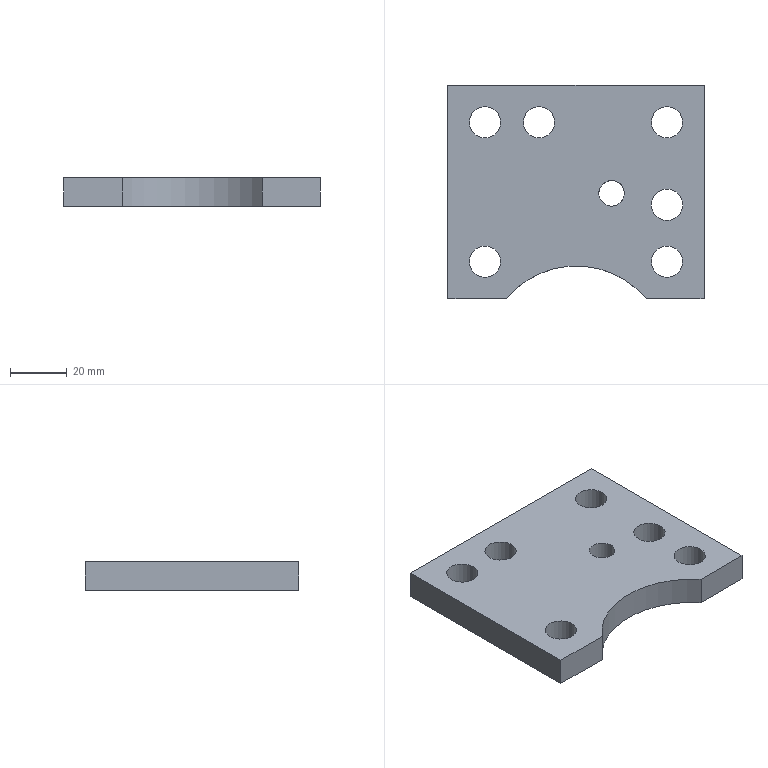Part | STEP file | PN_0043_id890_x_t | 1 solid | 15 faces | box 90 x 75 x 10 mm | volume 57234 mm3 | cylinder 8 | plane 7 | commonest cylinder face diameters 11 x6 9 x1 64 x1
STEP:
#1=CARTESIAN_POINT('',(-219.571,-141.5,105.));
#2=VERTEX_POINT('',#1);
#3=CARTESIAN_POINT('',(-219.571,-141.5,95.));
#4=VERTEX_POINT('',#3);
#5=CARTESIAN_POINT('',(-219.571,-141.5,96.5));
#6=DIRECTION('',(0.,0.,-1.));
#7=VECTOR('',#6,1.);
#8=LINE('',#5,#7);
#9=EDGE_CURVE('',#2,#4,#8,.T.);
#10=ORIENTED_EDGE('',*,*,#9,.F.);
#11=CARTESIAN_POINT('',(-240.086,-141.5,105.));
#12=VERTEX_POINT('',#11);
#13=CARTESIAN_POINT('',(-207.586,-141.5,105.));
#14=DIRECTION('',(-1.,0.,0.));
#15=VECTOR('',#14,1.);
#16=LINE('',#13,#15);
#17=EDGE_CURVE('',#2,#12,#16,.T.);
#18=ORIENTED_EDGE('',*,*,#17,.T.);
#19=CARTESIAN_POINT('',(-240.086,-141.5,95.));
#20=VERTEX_POINT('',#19);
#21=CARTESIAN_POINT('',(-240.086,-141.5,105.));
#22=DIRECTION('',(0.,0.,1.));
#23=VECTOR('',#22,1.);
#24=LINE('',#21,#23);
#25=EDGE_CURVE('',#20,#12,#24,.T.);
#26=ORIENTED_EDGE('',*,*,#25,.F.);
#27=CARTESIAN_POINT('',(-207.586,-141.5,95.));
#28=DIRECTION('',(1.,0.,0.));
#29=VECTOR('',#28,1.);
#30=LINE('',#27,#29);
#31=EDGE_CURVE('',#20,#4,#30,.T.);
#32=ORIENTED_EDGE('',*,*,#31,.T.);
#33=EDGE_LOOP('',(#10,#18,#26,#32));
#34=FACE_OUTER_BOUND('',#33,.T.);
#35=CARTESIAN_POINT('',(-207.586,-141.5,105.));
#36=DIRECTION('',(0.,-1.,0.));
#37=DIRECTION('',(0.,0.,-1.));
#38=AXIS2_PLACEMENT_3D('',#35,#36,#37);
#39=PLANE('',#38);
#40=ADVANCED_FACE('',(#34),#39,.T.);
#41=CARTESIAN_POINT('',(-221.586,-79.5,105.));
#42=VERTEX_POINT('',#41);
#43=CARTESIAN_POINT('',(-227.086,-79.5,105.));
#44=DIRECTION('',(0.,0.,1.));
#45=DIRECTION('',(1.,0.,0.));
#46=AXIS2_PLACEMENT_3D('',#43,#44,#45);
#47=CIRCLE('',#46,5.5);
#48=EDGE_CURVE('',#42,#42,#47,.T.);
#49=ORIENTED_EDGE('',*,*,#48,.F.);
#50=EDGE_LOOP('',(#49));
#51=FACE_BOUND('',#50,.T.);
#52=CARTESIAN_POINT('',(-202.586,-79.5,105.));
#53=VERTEX_POINT('',#52);
#54=CARTESIAN_POINT('',(-208.086,-79.5,105.));
#55=DIRECTION('',(0.,0.,-1.));
#56=DIRECTION('',(1.,0.,0.));
#57=AXIS2_PLACEMENT_3D('',#54,#55,#56);
#58=CIRCLE('',#57,5.5);
#59=EDGE_CURVE('',#53,#53,#58,.T.);
#60=ORIENTED_EDGE('',*,*,#59,.T.);
#61=EDGE_LOOP('',(#60));
#62=FACE_BOUND('',#61,.T.);
#63=CARTESIAN_POINT('',(-168.586,-79.5,105.));
#64=VERTEX_POINT('',#63);
#65=CARTESIAN_POINT('',(-163.086,-79.5,105.));
#66=DIRECTION('',(0.,0.,-1.));
#67=DIRECTION('',(-1.,0.,0.));
#68=AXIS2_PLACEMENT_3D('',#65,#66,#67);
#69=CIRCLE('',#68,5.5);
#70=EDGE_CURVE('',#64,#64,#69,.T.);
#71=ORIENTED_EDGE('',*,*,#70,.T.);
#72=EDGE_LOOP('',(#71));
#73=FACE_BOUND('',#72,.T.);
#74=CARTESIAN_POINT('',(-221.586,-128.5,105.));
#75=VERTEX_POINT('',#74);
#76=CARTESIAN_POINT('',(-227.086,-128.5,105.));
#77=DIRECTION('',(0.,0.,-1.));
#78=DIRECTION('',(1.,0.,0.));
#79=AXIS2_PLACEMENT_3D('',#76,#77,#78);
#80=CIRCLE('',#79,5.5);
#81=EDGE_CURVE('',#75,#75,#80,.T.);
#82=ORIENTED_EDGE('',*,*,#81,.T.);
#83=EDGE_LOOP('',(#82));
#84=FACE_BOUND('',#83,.T.);
#85=CARTESIAN_POINT('',(-168.586,-108.5,105.));
#86=VERTEX_POINT('',#85);
#87=CARTESIAN_POINT('',(-163.086,-108.5,105.));
#88=DIRECTION('',(0.,0.,-1.));
#89=DIRECTION('',(-1.,0.,0.));
#90=AXIS2_PLACEMENT_3D('',#87,#88,#89);
#91=CIRCLE('',#90,5.5);
#92=EDGE_CURVE('',#86,#86,#91,.T.);
#93=ORIENTED_EDGE('',*,*,#92,.T.);
#94=EDGE_LOOP('',(#93));
#95=FACE_BOUND('',#94,.T.);
#96=CARTESIAN_POINT('',(-168.586,-128.5,105.));
#97=VERTEX_POINT('',#96);
#98=CARTESIAN_POINT('',(-163.086,-128.5,105.));
#99=DIRECTION('',(0.,0.,1.));
#100=DIRECTION('',(-1.,0.,0.));
#101=AXIS2_PLACEMENT_3D('',#98,#99,#100);
#102=CIRCLE('',#101,5.5);
#103=EDGE_CURVE('',#97,#97,#102,.T.);
#104=ORIENTED_EDGE('',*,*,#103,.F.);
#105=EDGE_LOOP('',(#104));
#106=FACE_BOUND('',#105,.T.);
#107=CARTESIAN_POINT('',(-182.586,-100.,105.));
#108=VERTEX_POINT('',#107);
#109=CARTESIAN_POINT('',(-182.586,-104.5,105.));
#110=DIRECTION('',(0.,0.,-1.));
#111=DIRECTION('',(0.,1.,0.));
#112=AXIS2_PLACEMENT_3D('',#109,#110,#111);
#113=CIRCLE('',#112,4.5);
#114=EDGE_CURVE('',#108,#108,#113,.T.);
#115=ORIENTED_EDGE('',*,*,#114,.T.);
#116=EDGE_LOOP('',(#115));
#117=FACE_BOUND('',#116,.T.);
#118=CARTESIAN_POINT('',(-170.429,-141.5,105.));
#119=VERTEX_POINT('',#118);
#120=CARTESIAN_POINT('',(-195.,-162.,105.));
#121=DIRECTION('',(0.,0.,1.));
#122=DIRECTION('',(1.,0.,0.));
#123=AXIS2_PLACEMENT_3D('',#120,#121,#122);
#124=CIRCLE('',#123,32.);
#125=EDGE_CURVE('',#119,#2,#124,.T.);
#126=ORIENTED_EDGE('',*,*,#125,.F.);
#127=CARTESIAN_POINT('',(-150.086,-141.5,105.));
#128=VERTEX_POINT('',#127);
#129=CARTESIAN_POINT('',(-207.586,-141.5,105.));
#130=DIRECTION('',(-1.,0.,0.));
#131=VECTOR('',#130,1.);
#132=LINE('',#129,#131);
#133=EDGE_CURVE('',#128,#119,#132,.T.);
#134=ORIENTED_EDGE('',*,*,#133,.F.);
#135=CARTESIAN_POINT('',(-150.086,-66.5,105.));
#136=VERTEX_POINT('',#135);
#137=CARTESIAN_POINT('',(-150.086,-99.,105.));
#138=DIRECTION('',(0.,-1.,0.));
#139=VECTOR('',#138,1.);
#140=LINE('',#137,#139);
#141=EDGE_CURVE('',#136,#128,#140,.T.);
#142=ORIENTED_EDGE('',*,*,#141,.F.);
#143=CARTESIAN_POINT('',(-240.086,-66.5,105.));
#144=VERTEX_POINT('',#143);
#145=CARTESIAN_POINT('',(-207.586,-66.5,105.));
#146=DIRECTION('',(1.,0.,0.));
#147=VECTOR('',#146,1.);
#148=LINE('',#145,#147);
#149=EDGE_CURVE('',#144,#136,#148,.T.);
#150=ORIENTED_EDGE('',*,*,#149,.F.);
#151=CARTESIAN_POINT('',(-240.086,-99.,105.));
#152=DIRECTION('',(0.,1.,0.));
#153=VECTOR('',#152,1.);
#154=LINE('',#151,#153);
#155=EDGE_CURVE('',#12,#144,#154,.T.);
#156=ORIENTED_EDGE('',*,*,#155,.F.);
#157=ORIENTED_EDGE('',*,*,#17,.F.);
#158=EDGE_LOOP('',(#126,#134,#142,#150,#156,#157));
#159=FACE_BOUND('',#158,.T.);
#160=CARTESIAN_POINT('',(-119.811,64.,105.));
#161=DIRECTION('',(0.,0.,1.));
#162=DIRECTION('',(1.,0.,0.));
#163=AXIS2_PLACEMENT_3D('',#160,#161,#162);
#164=PLANE('',#163);
#165=ADVANCED_FACE('',(#51,#62,#73,#84,#95,#106,#117,#159),#164,.T.);
#166=CARTESIAN_POINT('',(-170.429,-141.5,95.));
#167=VERTEX_POINT('',#166);
#168=CARTESIAN_POINT('',(-170.429,-141.5,96.5));
#169=DIRECTION('',(0.,0.,1.));
#170=VECTOR('',#169,1.);
#171=LINE('',#168,#170);
#172=EDGE_CURVE('',#167,#119,#171,.T.);
#173=ORIENTED_EDGE('',*,*,#172,.F.);
#174=CARTESIAN_POINT('',(-150.086,-141.5,95.));
#175=VERTEX_POINT('',#174);
#176=CARTESIAN_POINT('',(-207.586,-141.5,95.));
#177=DIRECTION('',(1.,0.,0.));
#178=VECTOR('',#177,1.);
#179=LINE('',#176,#178);
#180=EDGE_CURVE('',#167,#175,#179,.T.);
#181=ORIENTED_EDGE('',*,*,#180,.T.);
#182=CARTESIAN_POINT('',(-150.086,-141.5,105.));
#183=DIRECTION('',(0.,0.,1.));
#184=VECTOR('',#183,1.);
#185=LINE('',#182,#184);
#186=EDGE_CURVE('',#175,#128,#185,.T.);
#187=ORIENTED_EDGE('',*,*,#186,.T.);
#188=ORIENTED_EDGE('',*,*,#133,.T.);
#189=EDGE_LOOP('',(#173,#181,#187,#188));
#190=FACE_OUTER_BOUND('',#189,.T.);
#191=CARTESIAN_POINT('',(-207.586,-141.5,105.));
#192=DIRECTION('',(0.,-1.,0.));
#193=DIRECTION('',(0.,0.,-1.));
#194=AXIS2_PLACEMENT_3D('',#191,#192,#193);
#195=PLANE('',#194);
#196=ADVANCED_FACE('',(#190),#195,.T.);
#197=ORIENTED_EDGE('',*,*,#25,.T.);
#198=ORIENTED_EDGE('',*,*,#155,.T.);
#199=CARTESIAN_POINT('',(-240.086,-66.5,95.));
#200=VERTEX_POINT('',#199);
#201=CARTESIAN_POINT('',(-240.086,-66.5,105.));
#202=DIRECTION('',(0.,0.,1.));
#203=VECTOR('',#202,1.);
#204=LINE('',#201,#203);
#205=EDGE_CURVE('',#200,#144,#204,.T.);
#206=ORIENTED_EDGE('',*,*,#205,.F.);
#207=CARTESIAN_POINT('',(-240.086,-99.,95.));
#208=DIRECTION('',(0.,-1.,0.));
#209=VECTOR('',#208,1.);
#210=LINE('',#207,#209);
#211=EDGE_CURVE('',#200,#20,#210,.T.);
#212=ORIENTED_EDGE('',*,*,#211,.T.);
#213=EDGE_LOOP('',(#197,#198,#206,#212));
#214=FACE_OUTER_BOUND('',#213,.T.);
#215=CARTESIAN_POINT('',(-240.086,-99.,105.));
#216=DIRECTION('',(-1.,0.,0.));
#217=DIRECTION('',(0.,0.,1.));
#218=AXIS2_PLACEMENT_3D('',#215,#216,#217);
#219=PLANE('',#218);
#220=ADVANCED_FACE('',(#214),#219,.T.);
#221=ORIENTED_EDGE('',*,*,#205,.T.);
#222=ORIENTED_EDGE('',*,*,#149,.T.);
#223=CARTESIAN_POINT('',(-150.086,-66.5,95.));
#224=VERTEX_POINT('',#223);
#225=CARTESIAN_POINT('',(-150.086,-66.5,105.));
#226=DIRECTION('',(0.,0.,1.));
#227=VECTOR('',#226,1.);
#228=LINE('',#225,#227);
#229=EDGE_CURVE('',#224,#136,#228,.T.);
#230=ORIENTED_EDGE('',*,*,#229,.F.);
#231=CARTESIAN_POINT('',(-207.586,-66.5,95.));
#232=DIRECTION('',(-1.,0.,0.));
#233=VECTOR('',#232,1.);
#234=LINE('',#231,#233);
#235=EDGE_CURVE('',#224,#200,#234,.T.);
#236=ORIENTED_EDGE('',*,*,#235,.T.);
#237=EDGE_LOOP('',(#221,#222,#230,#236));
#238=FACE_OUTER_BOUND('',#237,.T.);
#239=CARTESIAN_POINT('',(-207.586,-66.5,105.));
#240=DIRECTION('',(0.,1.,0.));
#241=DIRECTION('',(0.,0.,1.));
#242=AXIS2_PLACEMENT_3D('',#239,#240,#241);
#243=PLANE('',#242);
#244=ADVANCED_FACE('',(#238),#243,.T.);
#245=CARTESIAN_POINT('',(-221.586,-79.5,95.));
#246=VERTEX_POINT('',#245);
#247=CARTESIAN_POINT('',(-227.086,-79.5,95.));
#248=DIRECTION('',(0.,0.,-1.));
#249=DIRECTION('',(1.,0.,0.));
#250=AXIS2_PLACEMENT_3D('',#247,#248,#249);
#251=CIRCLE('',#250,5.5);
#252=EDGE_CURVE('',#246,#246,#251,.T.);
#253=ORIENTED_EDGE('',*,*,#252,.F.);
#254=EDGE_LOOP('',(#253));
#255=FACE_BOUND('',#254,.T.);
#256=CARTESIAN_POINT('',(-202.586,-79.5,95.));
#257=VERTEX_POINT('',#256);
#258=CARTESIAN_POINT('',(-208.086,-79.5,95.));
#259=DIRECTION('',(0.,0.,1.));
#260=DIRECTION('',(1.,0.,0.));
#261=AXIS2_PLACEMENT_3D('',#258,#259,#260);
#262=CIRCLE('',#261,5.5);
#263=EDGE_CURVE('',#257,#257,#262,.T.);
#264=ORIENTED_EDGE('',*,*,#263,.T.);
#265=EDGE_LOOP('',(#264));
#266=FACE_BOUND('',#265,.T.);
#267=CARTESIAN_POINT('',(-157.586,-79.5,95.));
#268=VERTEX_POINT('',#267);
#269=CARTESIAN_POINT('',(-163.086,-79.5,95.));
#270=DIRECTION('',(0.,0.,-1.));
#271=DIRECTION('',(1.,0.,0.));
#272=AXIS2_PLACEMENT_3D('',#269,#270,#271);
#273=CIRCLE('',#272,5.5);
#274=EDGE_CURVE('',#268,#268,#273,.T.);
#275=ORIENTED_EDGE('',*,*,#274,.F.);
#276=EDGE_LOOP('',(#275));
#277=FACE_BOUND('',#276,.T.);
#278=CARTESIAN_POINT('',(-221.586,-128.5,95.));
#279=VERTEX_POINT('',#278);
#280=CARTESIAN_POINT('',(-227.086,-128.5,95.));
#281=DIRECTION('',(0.,0.,-1.));
#282=DIRECTION('',(1.,0.,0.));
#283=AXIS2_PLACEMENT_3D('',#280,#281,#282);
#284=CIRCLE('',#283,5.5);
#285=EDGE_CURVE('',#279,#279,#284,.T.);
#286=ORIENTED_EDGE('',*,*,#285,.F.);
#287=EDGE_LOOP('',(#286));
#288=FACE_BOUND('',#287,.T.);
#289=CARTESIAN_POINT('',(-168.586,-108.5,95.));
#290=VERTEX_POINT('',#289);
#291=CARTESIAN_POINT('',(-163.086,-108.5,95.));
#292=DIRECTION('',(0.,0.,1.));
#293=DIRECTION('',(-1.,0.,0.));
#294=AXIS2_PLACEMENT_3D('',#291,#292,#293);
#295=CIRCLE('',#294,5.5);
#296=EDGE_CURVE('',#290,#290,#295,.T.);
#297=ORIENTED_EDGE('',*,*,#296,.T.);
#298=EDGE_LOOP('',(#297));
#299=FACE_BOUND('',#298,.T.);
#300=CARTESIAN_POINT('',(-157.586,-128.5,95.));
#301=VERTEX_POINT('',#300);
#302=CARTESIAN_POINT('',(-163.086,-128.5,95.));
#303=DIRECTION('',(0.,0.,-1.));
#304=DIRECTION('',(1.,0.,0.));
#305=AXIS2_PLACEMENT_3D('',#302,#303,#304);
#306=CIRCLE('',#305,5.5);
#307=EDGE_CURVE('',#301,#301,#306,.T.);
#308=ORIENTED_EDGE('',*,*,#307,.F.);
#309=EDGE_LOOP('',(#308));
#310=FACE_BOUND('',#309,.T.);
#311=CARTESIAN_POINT('',(-178.086,-104.5,95.));
#312=VERTEX_POINT('',#311);
#313=CARTESIAN_POINT('',(-182.586,-104.5,95.));
#314=DIRECTION('',(0.,0.,-1.));
#315=DIRECTION('',(1.,0.,0.));
#316=AXIS2_PLACEMENT_3D('',#313,#314,#315);
#317=CIRCLE('',#316,4.5);
#318=EDGE_CURVE('',#312,#312,#317,.T.);
#319=ORIENTED_EDGE('',*,*,#318,.F.);
#320=EDGE_LOOP('',(#319));
#321=FACE_BOUND('',#320,.T.);
#322=CARTESIAN_POINT('',(-195.,-162.,95.));
#323=DIRECTION('',(0.,0.,-1.));
#324=DIRECTION('',(1.,0.,0.));
#325=AXIS2_PLACEMENT_3D('',#322,#323,#324);
#326=CIRCLE('',#325,32.);
#327=EDGE_CURVE('',#4,#167,#326,.T.);
#328=ORIENTED_EDGE('',*,*,#327,.F.);
#329=ORIENTED_EDGE('',*,*,#31,.F.);
#330=ORIENTED_EDGE('',*,*,#211,.F.);
#331=ORIENTED_EDGE('',*,*,#235,.F.);
#332=CARTESIAN_POINT('',(-150.086,-99.,95.));
#333=DIRECTION('',(0.,1.,0.));
#334=VECTOR('',#333,1.);
#335=LINE('',#332,#334);
#336=EDGE_CURVE('',#175,#224,#335,.T.);
#337=ORIENTED_EDGE('',*,*,#336,.F.);
#338=ORIENTED_EDGE('',*,*,#180,.F.);
#339=EDGE_LOOP('',(#328,#329,#330,#331,#337,#338));
#340=FACE_BOUND('',#339,.T.);
#341=CARTESIAN_POINT('',(-119.811,64.,95.));
#342=DIRECTION('',(0.,0.,1.));
#343=DIRECTION('',(1.,0.,0.));
#344=AXIS2_PLACEMENT_3D('',#341,#342,#343);
#345=PLANE('',#344);
#346=ADVANCED_FACE('',(#255,#266,#277,#288,#299,#310,#321,#340),#345,.F.);
#347=ORIENTED_EDGE('',*,*,#336,.T.);
#348=ORIENTED_EDGE('',*,*,#229,.T.);
#349=ORIENTED_EDGE('',*,*,#141,.T.);
#350=ORIENTED_EDGE('',*,*,#186,.F.);
#351=EDGE_LOOP('',(#347,#348,#349,#350));
#352=FACE_OUTER_BOUND('',#351,.T.);
#353=CARTESIAN_POINT('',(-150.086,-99.,105.));
#354=DIRECTION('',(1.,0.,0.));
#355=DIRECTION('',(0.,0.,-1.));
#356=AXIS2_PLACEMENT_3D('',#353,#354,#355);
#357=PLANE('',#356);
#358=ADVANCED_FACE('',(#352),#357,.T.);
#359=ORIENTED_EDGE('',*,*,#125,.T.);
#360=ORIENTED_EDGE('',*,*,#9,.T.);
#361=ORIENTED_EDGE('',*,*,#327,.T.);
#362=ORIENTED_EDGE('',*,*,#172,.T.);
#363=EDGE_LOOP('',(#359,#360,#361,#362));
#364=FACE_OUTER_BOUND('',#363,.T.);
#365=CARTESIAN_POINT('',(-195.,-162.,96.5));
#366=DIRECTION('',(0.,0.,-1.));
#367=DIRECTION('',(1.,0.,0.));
#368=AXIS2_PLACEMENT_3D('',#365,#366,#367);
#369=CYLINDRICAL_SURFACE('',#368,32.);
#370=ADVANCED_FACE('',(#364),#369,.F.);
#371=ORIENTED_EDGE('',*,*,#318,.T.);
#372=EDGE_LOOP('',(#371));
#373=FACE_BOUND('',#372,.T.);
#374=ORIENTED_EDGE('',*,*,#114,.F.);
#375=EDGE_LOOP('',(#374));
#376=FACE_BOUND('',#375,.T.);
#377=CARTESIAN_POINT('',(-182.586,-104.5,105.));
#378=DIRECTION('',(0.,0.,-1.));
#379=DIRECTION('',(0.,1.,0.));
#380=AXIS2_PLACEMENT_3D('',#377,#378,#379);
#381=CYLINDRICAL_SURFACE('',#380,4.5);
#382=ADVANCED_FACE('',(#373,#376),#381,.F.);
#383=ORIENTED_EDGE('',*,*,#307,.T.);
#384=EDGE_LOOP('',(#383));
#385=FACE_BOUND('',#384,.T.);
#386=ORIENTED_EDGE('',*,*,#103,.T.);
#387=EDGE_LOOP('',(#386));
#388=FACE_BOUND('',#387,.T.);
#389=CARTESIAN_POINT('',(-163.086,-128.5,105.));
#390=DIRECTION('',(0.,0.,-1.));
#391=DIRECTION('',(-1.,0.,0.));
#392=AXIS2_PLACEMENT_3D('',#389,#390,#391);
#393=CYLINDRICAL_SURFACE('',#392,5.5);
#394=ADVANCED_FACE('',(#385,#388),#393,.F.);
#395=ORIENTED_EDGE('',*,*,#296,.F.);
#396=EDGE_LOOP('',(#395));
#397=FACE_BOUND('',#396,.T.);
#398=ORIENTED_EDGE('',*,*,#92,.F.);
#399=EDGE_LOOP('',(#398));
#400=FACE_BOUND('',#399,.T.);
#401=CARTESIAN_POINT('',(-163.086,-108.5,105.));
#402=DIRECTION('',(0.,0.,-1.));
#403=DIRECTION('',(-1.,0.,0.));
#404=AXIS2_PLACEMENT_3D('',#401,#402,#403);
#405=CYLINDRICAL_SURFACE('',#404,5.5);
#406=ADVANCED_FACE('',(#397,#400),#405,.F.);
#407=ORIENTED_EDGE('',*,*,#285,.T.);
#408=EDGE_LOOP('',(#407));
#409=FACE_BOUND('',#408,.T.);
#410=ORIENTED_EDGE('',*,*,#81,.F.);
#411=EDGE_LOOP('',(#410));
#412=FACE_BOUND('',#411,.T.);
#413=CARTESIAN_POINT('',(-227.086,-128.5,105.));
#414=DIRECTION('',(0.,0.,-1.));
#415=DIRECTION('',(1.,0.,0.));
#416=AXIS2_PLACEMENT_3D('',#413,#414,#415);
#417=CYLINDRICAL_SURFACE('',#416,5.5);
#418=ADVANCED_FACE('',(#409,#412),#417,.F.);
#419=ORIENTED_EDGE('',*,*,#274,.T.);
#420=EDGE_LOOP('',(#419));
#421=FACE_BOUND('',#420,.T.);
#422=ORIENTED_EDGE('',*,*,#70,.F.);
#423=EDGE_LOOP('',(#422));
#424=FACE_BOUND('',#423,.T.);
#425=CARTESIAN_POINT('',(-163.086,-79.5,105.));
#426=DIRECTION('',(0.,0.,-1.));
#427=DIRECTION('',(-1.,0.,0.));
#428=AXIS2_PLACEMENT_3D('',#425,#426,#427);
#429=CYLINDRICAL_SURFACE('',#428,5.5);
#430=ADVANCED_FACE('',(#421,#424),#429,.F.);
#431=ORIENTED_EDGE('',*,*,#263,.F.);
#432=EDGE_LOOP('',(#431));
#433=FACE_BOUND('',#432,.T.);
#434=ORIENTED_EDGE('',*,*,#59,.F.);
#435=EDGE_LOOP('',(#434));
#436=FACE_BOUND('',#435,.T.);
#437=CARTESIAN_POINT('',(-208.086,-79.5,105.));
#438=DIRECTION('',(0.,0.,-1.));
#439=DIRECTION('',(1.,0.,0.));
#440=AXIS2_PLACEMENT_3D('',#437,#438,#439);
#441=CYLINDRICAL_SURFACE('',#440,5.5);
#442=ADVANCED_FACE('',(#433,#436),#441,.F.);
#443=ORIENTED_EDGE('',*,*,#252,.T.);
#444=EDGE_LOOP('',(#443));
#445=FACE_BOUND('',#444,.T.);
#446=ORIENTED_EDGE('',*,*,#48,.T.);
#447=EDGE_LOOP('',(#446));
#448=FACE_BOUND('',#447,.T.);
#449=CARTESIAN_POINT('',(-227.086,-79.5,105.));
#450=DIRECTION('',(0.,0.,-1.));
#451=DIRECTION('',(1.,0.,0.));
#452=AXIS2_PLACEMENT_3D('',#449,#450,#451);
#453=CYLINDRICAL_SURFACE('',#452,5.5);
#454=ADVANCED_FACE('',(#445,#448),#453,.F.);
#455=CLOSED_SHELL('',(#40,#165,#196,#220,#244,#346,#358,#370,#382,#394,#406,#418,#430,#442,#454));
#456=MANIFOLD_SOLID_BREP('',#455);
#457=(LENGTH_UNIT()NAMED_UNIT(*)SI_UNIT(.MILLI.,.METRE.));
#458=UNCERTAINTY_MEASURE_WITH_UNIT(LENGTH_MEASURE(0.00002),#457,'','');
#459=(NAMED_UNIT(*)PLANE_ANGLE_UNIT()SI_UNIT($,.RADIAN.));
#460=PLANE_ANGLE_MEASURE_WITH_UNIT(PLANE_ANGLE_MEASURE(0.01745),#459);
#461=DIMENSIONAL_EXPONENTS(0.,0.,0.,0.,0.,0.,0.);
#462=(CONVERSION_BASED_UNIT('DEGREE',#460)NAMED_UNIT(#461)PLANE_ANGLE_UNIT());
#463=(NAMED_UNIT(*)SI_UNIT($,.STERADIAN.)SOLID_ANGLE_UNIT());
#464=(GEOMETRIC_REPRESENTATION_CONTEXT(3)GLOBAL_UNCERTAINTY_ASSIGNED_CONTEXT((#458))GLOBAL_UNIT_ASSIGNED_CONTEXT((#457,#462,#463))REPRESENTATION_CONTEXT('',''));
#465=ADVANCED_BREP_SHAPE_REPRESENTATION('',(#456),#464);